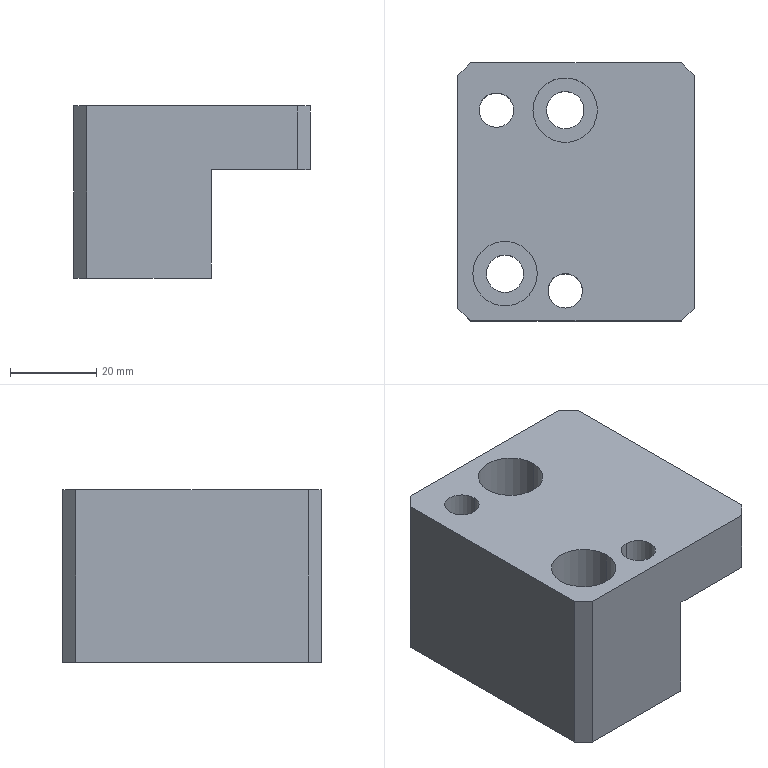Part | STEP file | 1_id1458_x_t | 1 solid | 29 faces | box 55 x 60 x 40 mm | volume 83432 mm3 | plane 15 | cylinder 14 | commonest cylinder face diameters 8 x4 8.7 x4 15 x4 12.5 x2